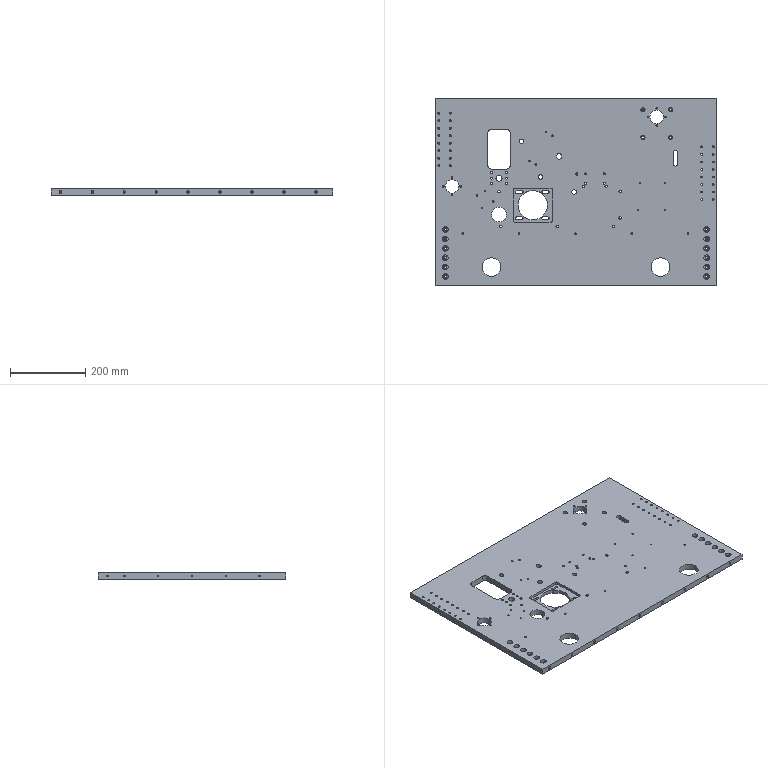Part | STEP file | MT-COMBO-119-S002 | 1 solid | 473 faces | box 750 x 500 x 16 mm | volume 5589140 mm3 | cylinder 334 | cone 84 | plane 55 | commonest cylinder face diameters 4.2 x74 5 x64 6.6 x32 9 x24 15 x24 5.5 x20